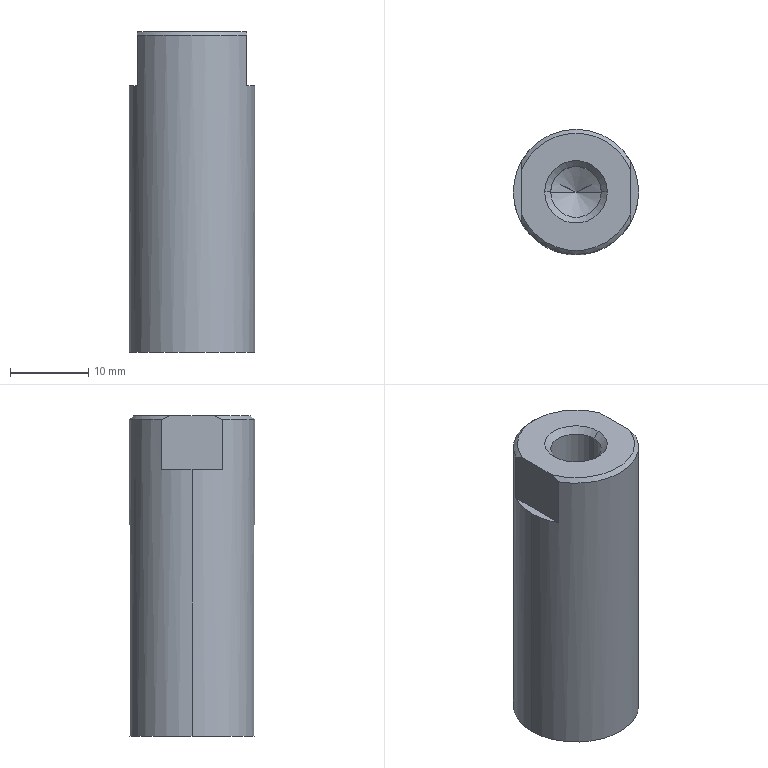Part | NX | features BREP 1 | 1 solid | 16 faces | box 16 x 16 x 41 mm | volume 7697 mm3 | cone 6 | plane 6 | cylinder 4 | commonest cylinder face diameters 6.47 x2 16 x2
STEP:
#1=CARTESIAN_POINT('',(7.,3.873,0.1));
#2=VERTEX_POINT('',#1);
#3=CARTESIAN_POINT('',(8.,0.,0.1));
#4=VERTEX_POINT('',#3);
#5=CARTESIAN_POINT('',(0.,0.,0.1));
#6=DIRECTION('',(0.,0.,-1.));
#7=DIRECTION('',(-1.,0.,0.));
#8=AXIS2_PLACEMENT_3D('',#5,#6,#7);
#9=CIRCLE('',#8,8.);
#10=EDGE_CURVE('',#2,#4,#9,.T.);
#11=ORIENTED_EDGE('',*,*,#10,.T.);
#12=CARTESIAN_POINT('',(8.,0.,-34.));
#13=VERTEX_POINT('',#12);
#14=CARTESIAN_POINT('',(8.,0.,-13.75));
#15=DIRECTION('',(0.,0.,-1.));
#16=VECTOR('',#15,1000.);
#17=LINE('',#14,#16);
#18=EDGE_CURVE('',#4,#13,#17,.T.);
#19=ORIENTED_EDGE('',*,*,#18,.T.);
#20=CARTESIAN_POINT('',(-8.,0.,-34.));
#21=VERTEX_POINT('',#20);
#22=CARTESIAN_POINT('',(0.,0.,-34.));
#23=DIRECTION('',(0.,0.,1.));
#24=DIRECTION('',(-1.,0.,0.));
#25=AXIS2_PLACEMENT_3D('',#22,#23,#24);
#26=CIRCLE('',#25,8.);
#27=EDGE_CURVE('',#13,#21,#26,.T.);
#28=ORIENTED_EDGE('',*,*,#27,.T.);
#29=CARTESIAN_POINT('',(-8.,0.,0.1));
#30=VERTEX_POINT('',#29);
#31=CARTESIAN_POINT('',(-8.,0.,-13.75));
#32=DIRECTION('',(0.,0.,-1.));
#33=VECTOR('',#32,1000.);
#34=LINE('',#31,#33);
#35=EDGE_CURVE('',#30,#21,#34,.T.);
#36=ORIENTED_EDGE('',*,*,#35,.F.);
#37=CARTESIAN_POINT('',(-7.,3.873,0.1));
#38=VERTEX_POINT('',#37);
#39=CARTESIAN_POINT('',(0.,0.,0.1));
#40=DIRECTION('',(0.,0.,-1.));
#41=DIRECTION('',(-1.,0.,0.));
#42=AXIS2_PLACEMENT_3D('',#39,#40,#41);
#43=CIRCLE('',#42,8.);
#44=EDGE_CURVE('',#30,#38,#43,.T.);
#45=ORIENTED_EDGE('',*,*,#44,.T.);
#46=CARTESIAN_POINT('',(-7.,3.873,6.5));
#47=VERTEX_POINT('',#46);
#48=CARTESIAN_POINT('',(-7.,3.873,-13.75));
#49=DIRECTION('',(0.,0.,1.));
#50=VECTOR('',#49,1000.);
#51=LINE('',#48,#50);
#52=EDGE_CURVE('',#38,#47,#51,.T.);
#53=ORIENTED_EDGE('',*,*,#52,.T.);
#54=CARTESIAN_POINT('',(7.,3.873,6.5));
#55=VERTEX_POINT('',#54);
#56=CARTESIAN_POINT('',(0.,0.,6.5));
#57=DIRECTION('',(0.,0.,-1.));
#58=DIRECTION('',(-1.,0.,0.));
#59=AXIS2_PLACEMENT_3D('',#56,#57,#58);
#60=CIRCLE('',#59,8.);
#61=EDGE_CURVE('',#47,#55,#60,.T.);
#62=ORIENTED_EDGE('',*,*,#61,.T.);
#63=CARTESIAN_POINT('',(7.,3.873,-13.75));
#64=DIRECTION('',(0.,0.,-1.));
#65=VECTOR('',#64,1000.);
#66=LINE('',#63,#65);
#67=EDGE_CURVE('',#55,#2,#66,.T.);
#68=ORIENTED_EDGE('',*,*,#67,.T.);
#69=EDGE_LOOP('',(#11,#19,#28,#36,#45,#53,#62,#68));
#70=FACE_BOUND('',#69,.T.);
#71=CARTESIAN_POINT('',(0.,0.,-13.75));
#72=DIRECTION('',(0.,0.,-1.));
#73=DIRECTION('',(-1.,0.,0.));
#74=AXIS2_PLACEMENT_3D('',#71,#72,#73);
#75=CYLINDRICAL_SURFACE('',#74,8.);
#76=ADVANCED_FACE('',(#70),#75,.T.);
#77=CARTESIAN_POINT('',(-3.235,0.,6.235));
#78=VERTEX_POINT('',#77);
#79=CARTESIAN_POINT('',(3.235,0.,6.235));
#80=VERTEX_POINT('',#79);
#81=CARTESIAN_POINT('',(0.,0.,6.235));
#82=DIRECTION('',(0.,0.,1.));
#83=DIRECTION('',(0.,1.,0.));
#84=AXIS2_PLACEMENT_3D('',#81,#82,#83);
#85=CIRCLE('',#84,3.235);
#86=EDGE_CURVE('',#78,#80,#85,.T.);
#87=ORIENTED_EDGE('',*,*,#86,.F.);
#88=CARTESIAN_POINT('',(-4.,0.,7.));
#89=VERTEX_POINT('',#88);
#90=CARTESIAN_POINT('',(-4.,0.,7.));
#91=DIRECTION('',(-0.7071,0.,0.7071));
#92=VECTOR('',#91,1000.);
#93=LINE('',#90,#92);
#94=EDGE_CURVE('',#89,#78,#93,.F.);
#95=ORIENTED_EDGE('',*,*,#94,.F.);
#96=CARTESIAN_POINT('',(4.,0.,7.));
#97=VERTEX_POINT('',#96);
#98=CARTESIAN_POINT('',(0.,0.,7.));
#99=DIRECTION('',(0.,0.,-1.));
#100=DIRECTION('',(1.,0.,0.));
#101=AXIS2_PLACEMENT_3D('',#98,#99,#100);
#102=CIRCLE('',#101,4.);
#103=EDGE_CURVE('',#97,#89,#102,.T.);
#104=ORIENTED_EDGE('',*,*,#103,.F.);
#105=CARTESIAN_POINT('',(4.,0.,7.));
#106=DIRECTION('',(0.7071,0.,0.7071));
#107=VECTOR('',#106,1000.);
#108=LINE('',#105,#107);
#109=EDGE_CURVE('',#97,#80,#108,.F.);
#110=ORIENTED_EDGE('',*,*,#109,.T.);
#111=EDGE_LOOP('',(#87,#95,#104,#110));
#112=FACE_BOUND('',#111,.T.);
#113=CARTESIAN_POINT('',(0.,0.,7.));
#114=DIRECTION('',(0.,0.,1.));
#115=DIRECTION('',(1.,0.,0.));
#116=AXIS2_PLACEMENT_3D('',#113,#114,#115);
#117=CONICAL_SURFACE('',#116,4.,0.7854);
#118=ADVANCED_FACE('',(#112),#117,.F.);
#119=ORIENTED_EDGE('',*,*,#86,.T.);
#120=CARTESIAN_POINT('',(3.235,0.,-6.5));
#121=VERTEX_POINT('',#120);
#122=CARTESIAN_POINT('',(3.235,0.,-0.1325));
#123=DIRECTION('',(0.,0.,-1.));
#124=VECTOR('',#123,1000.);
#125=LINE('',#122,#124);
#126=EDGE_CURVE('',#80,#121,#125,.T.);
#127=ORIENTED_EDGE('',*,*,#126,.T.);
#128=CARTESIAN_POINT('',(-3.235,0.,-6.5));
#129=VERTEX_POINT('',#128);
#130=CARTESIAN_POINT('',(0.,0.,-6.5));
#131=DIRECTION('',(0.,0.,1.));
#132=DIRECTION('',(-1.,0.,0.));
#133=AXIS2_PLACEMENT_3D('',#130,#131,#132);
#134=CIRCLE('',#133,3.235);
#135=EDGE_CURVE('',#129,#121,#134,.T.);
#136=ORIENTED_EDGE('',*,*,#135,.F.);
#137=CARTESIAN_POINT('',(-3.235,0.,-0.1325));
#138=DIRECTION('',(0.,0.,-1.));
#139=VECTOR('',#138,1000.);
#140=LINE('',#137,#139);
#141=EDGE_CURVE('',#78,#129,#140,.T.);
#142=ORIENTED_EDGE('',*,*,#141,.F.);
#143=EDGE_LOOP('',(#119,#127,#136,#142));
#144=FACE_BOUND('',#143,.T.);
#145=CARTESIAN_POINT('',(0.,0.,-0.1325));
#146=DIRECTION('',(0.,0.,-1.));
#147=DIRECTION('',(-1.,0.,0.));
#148=AXIS2_PLACEMENT_3D('',#145,#146,#147);
#149=CYLINDRICAL_SURFACE('',#148,3.235);
#150=ADVANCED_FACE('',(#144),#149,.F.);
#151=CARTESIAN_POINT('',(0.,0.,-8.368));
#152=VERTEX_POINT('',#151);
#153=CARTESIAN_POINT('',(3.235,0.,-6.5));
#154=DIRECTION('',(0.866,0.,0.5));
#155=VECTOR('',#154,1000.);
#156=LINE('',#153,#155);
#157=EDGE_CURVE('',#121,#152,#156,.F.);
#158=ORIENTED_EDGE('',*,*,#157,.T.);
#159=CARTESIAN_POINT('',(-3.235,0.,-6.5));
#160=DIRECTION('',(-0.866,0.,0.5));
#161=VECTOR('',#160,1000.);
#162=LINE('',#159,#161);
#163=EDGE_CURVE('',#129,#152,#162,.F.);
#164=ORIENTED_EDGE('',*,*,#163,.F.);
#165=ORIENTED_EDGE('',*,*,#135,.T.);
#166=EDGE_LOOP('',(#158,#164,#165));
#167=FACE_BOUND('',#166,.T.);
#168=CARTESIAN_POINT('',(0.,0.,-6.5));
#169=DIRECTION('',(0.,0.,1.));
#170=DIRECTION('',(1.,0.,0.));
#171=AXIS2_PLACEMENT_3D('',#168,#169,#170);
#172=CONICAL_SURFACE('',#171,3.235,1.047);
#173=ADVANCED_FACE('',(#167),#172,.F.);
#174=ORIENTED_EDGE('',*,*,#18,.F.);
#175=CARTESIAN_POINT('',(7.,-3.873,0.1));
#176=VERTEX_POINT('',#175);
#177=CARTESIAN_POINT('',(0.,0.,0.1));
#178=DIRECTION('',(0.,0.,-1.));
#179=DIRECTION('',(-1.,0.,0.));
#180=AXIS2_PLACEMENT_3D('',#177,#178,#179);
#181=CIRCLE('',#180,8.);
#182=EDGE_CURVE('',#4,#176,#181,.T.);
#183=ORIENTED_EDGE('',*,*,#182,.T.);
#184=CARTESIAN_POINT('',(7.,-3.873,6.5));
#185=VERTEX_POINT('',#184);
#186=CARTESIAN_POINT('',(7.,-3.873,-13.75));
#187=DIRECTION('',(0.,0.,1.));
#188=VECTOR('',#187,1000.);
#189=LINE('',#186,#188);
#190=EDGE_CURVE('',#176,#185,#189,.T.);
#191=ORIENTED_EDGE('',*,*,#190,.T.);
#192=CARTESIAN_POINT('',(-7.,-3.873,6.5));
#193=VERTEX_POINT('',#192);
#194=CARTESIAN_POINT('',(0.,0.,6.5));
#195=DIRECTION('',(0.,0.,-1.));
#196=DIRECTION('',(-1.,0.,0.));
#197=AXIS2_PLACEMENT_3D('',#194,#195,#196);
#198=CIRCLE('',#197,8.);
#199=EDGE_CURVE('',#185,#193,#198,.T.);
#200=ORIENTED_EDGE('',*,*,#199,.T.);
#201=CARTESIAN_POINT('',(-7.,-3.873,0.1));
#202=VERTEX_POINT('',#201);
#203=CARTESIAN_POINT('',(-7.,-3.873,-13.75));
#204=DIRECTION('',(0.,0.,-1.));
#205=VECTOR('',#204,1000.);
#206=LINE('',#203,#205);
#207=EDGE_CURVE('',#193,#202,#206,.T.);
#208=ORIENTED_EDGE('',*,*,#207,.T.);
#209=CARTESIAN_POINT('',(0.,0.,0.1));
#210=DIRECTION('',(0.,0.,-1.));
#211=DIRECTION('',(-1.,0.,0.));
#212=AXIS2_PLACEMENT_3D('',#209,#210,#211);
#213=CIRCLE('',#212,8.);
#214=EDGE_CURVE('',#202,#30,#213,.T.);
#215=ORIENTED_EDGE('',*,*,#214,.T.);
#216=ORIENTED_EDGE('',*,*,#35,.T.);
#217=CARTESIAN_POINT('',(0.,0.,-34.));
#218=DIRECTION('',(0.,0.,1.));
#219=DIRECTION('',(-1.,0.,0.));
#220=AXIS2_PLACEMENT_3D('',#217,#218,#219);
#221=CIRCLE('',#220,8.);
#222=EDGE_CURVE('',#21,#13,#221,.T.);
#223=ORIENTED_EDGE('',*,*,#222,.T.);
#224=EDGE_LOOP('',(#174,#183,#191,#200,#208,#215,#216,#223));
#225=FACE_BOUND('',#224,.T.);
#226=CARTESIAN_POINT('',(0.,0.,-13.75));
#227=DIRECTION('',(0.,0.,-1.));
#228=DIRECTION('',(-1.,0.,0.));
#229=AXIS2_PLACEMENT_3D('',#226,#227,#228);
#230=CYLINDRICAL_SURFACE('',#229,8.);
#231=ADVANCED_FACE('',(#225),#230,.T.);
#232=CARTESIAN_POINT('',(-7.,2.693,7.));
#233=VERTEX_POINT('',#232);
#234=CARTESIAN_POINT('',(-7.,2.693,7.));
#235=CARTESIAN_POINT('',(-7.,3.073,6.863));
#236=CARTESIAN_POINT('',(-7.,3.467,6.697));
#237=CARTESIAN_POINT('',(-7.,3.873,6.5));
#238=B_SPLINE_CURVE_WITH_KNOTS('',3,(#234,#235,#236,#237),.UNSPECIFIED.,.F.,.F.,(4,4),(0.,1.),.UNSPECIFIED.);
#239=EDGE_CURVE('',#47,#233,#238,.F.);
#240=ORIENTED_EDGE('',*,*,#239,.T.);
#241=CARTESIAN_POINT('',(7.,2.693,7.));
#242=VERTEX_POINT('',#241);
#243=CARTESIAN_POINT('',(0.,0.,7.));
#244=DIRECTION('',(0.,0.,-1.));
#245=DIRECTION('',(-1.,0.,0.));
#246=AXIS2_PLACEMENT_3D('',#243,#244,#245);
#247=CIRCLE('',#246,7.5);
#248=EDGE_CURVE('',#233,#242,#247,.T.);
#249=ORIENTED_EDGE('',*,*,#248,.T.);
#250=CARTESIAN_POINT('',(7.,3.873,6.5));
#251=CARTESIAN_POINT('',(7.,3.467,6.697));
#252=CARTESIAN_POINT('',(7.,3.073,6.863));
#253=CARTESIAN_POINT('',(7.,2.693,7.));
#254=B_SPLINE_CURVE_WITH_KNOTS('',3,(#250,#251,#252,#253),.UNSPECIFIED.,.F.,.F.,(4,4),(0.,1.),.UNSPECIFIED.);
#255=EDGE_CURVE('',#242,#55,#254,.F.);
#256=ORIENTED_EDGE('',*,*,#255,.T.);
#257=ORIENTED_EDGE('',*,*,#61,.F.);
#258=EDGE_LOOP('',(#240,#249,#256,#257));
#259=FACE_BOUND('',#258,.T.);
#260=CARTESIAN_POINT('',(0.,0.,6.5));
#261=DIRECTION('',(0.,0.,-1.));
#262=DIRECTION('',(-1.,0.,0.));
#263=AXIS2_PLACEMENT_3D('',#260,#261,#262);
#264=CONICAL_SURFACE('',#263,8.,0.7854);
#265=ADVANCED_FACE('',(#259),#264,.T.);
#266=CARTESIAN_POINT('',(-7.,-2.693,7.));
#267=VERTEX_POINT('',#266);
#268=CARTESIAN_POINT('',(-7.,-10.,7.));
#269=DIRECTION('',(0.,-1.,0.));
#270=VECTOR('',#269,1000.);
#271=LINE('',#268,#270);
#272=EDGE_CURVE('',#233,#267,#271,.T.);
#273=ORIENTED_EDGE('',*,*,#272,.F.);
#274=ORIENTED_EDGE('',*,*,#239,.F.);
#275=ORIENTED_EDGE('',*,*,#52,.F.);
#276=CARTESIAN_POINT('',(-7.,-10.,0.1));
#277=DIRECTION('',(0.,1.,0.));
#278=VECTOR('',#277,1000.);
#279=LINE('',#276,#278);
#280=EDGE_CURVE('',#202,#38,#279,.T.);
#281=ORIENTED_EDGE('',*,*,#280,.F.);
#282=ORIENTED_EDGE('',*,*,#207,.F.);
#283=CARTESIAN_POINT('',(-7.,-3.873,6.5));
#284=CARTESIAN_POINT('',(-7.,-3.467,6.697));
#285=CARTESIAN_POINT('',(-7.,-3.073,6.863));
#286=CARTESIAN_POINT('',(-7.,-2.693,7.));
#287=B_SPLINE_CURVE_WITH_KNOTS('',3,(#283,#284,#285,#286),.UNSPECIFIED.,.F.,.F.,(4,4),(0.,1.),.UNSPECIFIED.);
#288=EDGE_CURVE('',#267,#193,#287,.F.);
#289=ORIENTED_EDGE('',*,*,#288,.F.);
#290=EDGE_LOOP('',(#273,#274,#275,#281,#282,#289));
#291=FACE_BOUND('',#290,.T.);
#292=CARTESIAN_POINT('',(-7.,-10.,7.));
#293=DIRECTION('',(1.,0.,0.));
#294=DIRECTION('',(0.,1.,0.));
#295=AXIS2_PLACEMENT_3D('',#292,#293,#294);
#296=PLANE('',#295);
#297=ADVANCED_FACE('',(#291),#296,.F.);
#298=ORIENTED_EDGE('',*,*,#214,.F.);
#299=ORIENTED_EDGE('',*,*,#280,.T.);
#300=ORIENTED_EDGE('',*,*,#44,.F.);
#301=EDGE_LOOP('',(#298,#299,#300));
#302=FACE_BOUND('',#301,.T.);
#303=CARTESIAN_POINT('',(0.,0.,0.1));
#304=DIRECTION('',(0.,0.,1.));
#305=DIRECTION('',(1.,0.,0.));
#306=AXIS2_PLACEMENT_3D('',#303,#304,#305);
#307=PLANE('',#306);
#308=ADVANCED_FACE('',(#302),#307,.T.);
#309=ORIENTED_EDGE('',*,*,#288,.T.);
#310=ORIENTED_EDGE('',*,*,#199,.F.);
#311=CARTESIAN_POINT('',(7.,-2.693,7.));
#312=VERTEX_POINT('',#311);
#313=CARTESIAN_POINT('',(7.,-2.693,7.));
#314=CARTESIAN_POINT('',(7.,-3.073,6.863));
#315=CARTESIAN_POINT('',(7.,-3.467,6.697));
#316=CARTESIAN_POINT('',(7.,-3.873,6.5));
#317=B_SPLINE_CURVE_WITH_KNOTS('',3,(#313,#314,#315,#316),.UNSPECIFIED.,.F.,.F.,(4,4),(0.,1.),.UNSPECIFIED.);
#318=EDGE_CURVE('',#185,#312,#317,.F.);
#319=ORIENTED_EDGE('',*,*,#318,.T.);
#320=CARTESIAN_POINT('',(0.,0.,7.));
#321=DIRECTION('',(0.,0.,-1.));
#322=DIRECTION('',(-1.,0.,0.));
#323=AXIS2_PLACEMENT_3D('',#320,#321,#322);
#324=CIRCLE('',#323,7.5);
#325=EDGE_CURVE('',#312,#267,#324,.T.);
#326=ORIENTED_EDGE('',*,*,#325,.T.);
#327=EDGE_LOOP('',(#309,#310,#319,#326));
#328=FACE_BOUND('',#327,.T.);
#329=CARTESIAN_POINT('',(0.,0.,6.5));
#330=DIRECTION('',(0.,0.,-1.));
#331=DIRECTION('',(-1.,0.,0.));
#332=AXIS2_PLACEMENT_3D('',#329,#330,#331);
#333=CONICAL_SURFACE('',#332,8.,0.7854);
#334=ADVANCED_FACE('',(#328),#333,.T.);
#335=ORIENTED_EDGE('',*,*,#222,.F.);
#336=ORIENTED_EDGE('',*,*,#27,.F.);
#337=EDGE_LOOP('',(#335,#336));
#338=FACE_BOUND('',#337,.T.);
#339=CARTESIAN_POINT('',(0.,4.,-34.));
#340=DIRECTION('',(0.,0.,-1.));
#341=DIRECTION('',(0.,-1.,0.));
#342=AXIS2_PLACEMENT_3D('',#339,#340,#341);
#343=PLANE('',#342);
#344=ADVANCED_FACE('',(#338),#343,.T.);
#345=CARTESIAN_POINT('',(7.,3.75,7.));
#346=DIRECTION('',(0.,1.,0.));
#347=VECTOR('',#346,1000.);
#348=LINE('',#345,#347);
#349=EDGE_CURVE('',#312,#242,#348,.T.);
#350=ORIENTED_EDGE('',*,*,#349,.T.);
#351=ORIENTED_EDGE('',*,*,#248,.F.);
#352=ORIENTED_EDGE('',*,*,#272,.T.);
#353=ORIENTED_EDGE('',*,*,#325,.F.);
#354=EDGE_LOOP('',(#350,#351,#352,#353));
#355=FACE_BOUND('',#354,.T.);
#356=ORIENTED_EDGE('',*,*,#103,.T.);
#357=CARTESIAN_POINT('',(0.,0.,7.));
#358=DIRECTION('',(0.,0.,-1.));
#359=DIRECTION('',(1.,0.,0.));
#360=AXIS2_PLACEMENT_3D('',#357,#358,#359);
#361=CIRCLE('',#360,4.);
#362=EDGE_CURVE('',#89,#97,#361,.T.);
#363=ORIENTED_EDGE('',*,*,#362,.T.);
#364=EDGE_LOOP('',(#356,#363));
#365=FACE_BOUND('',#364,.T.);
#366=CARTESIAN_POINT('',(0.,3.75,7.));
#367=DIRECTION('',(0.,0.,1.));
#368=DIRECTION('',(1.,0.,0.));
#369=AXIS2_PLACEMENT_3D('',#366,#367,#368);
#370=PLANE('',#369);
#371=ADVANCED_FACE('',(#355,#365),#370,.T.);
#372=ORIENTED_EDGE('',*,*,#349,.F.);
#373=ORIENTED_EDGE('',*,*,#318,.F.);
#374=ORIENTED_EDGE('',*,*,#190,.F.);
#375=CARTESIAN_POINT('',(7.,10.,0.1));
#376=DIRECTION('',(0.,-1.,0.));
#377=VECTOR('',#376,1000.);
#378=LINE('',#375,#377);
#379=EDGE_CURVE('',#2,#176,#378,.T.);
#380=ORIENTED_EDGE('',*,*,#379,.F.);
#381=ORIENTED_EDGE('',*,*,#67,.F.);
#382=ORIENTED_EDGE('',*,*,#255,.F.);
#383=EDGE_LOOP('',(#372,#373,#374,#380,#381,#382));
#384=FACE_BOUND('',#383,.T.);
#385=CARTESIAN_POINT('',(7.,10.,7.));
#386=DIRECTION('',(-1.,0.,0.));
#387=DIRECTION('',(0.,0.,1.));
#388=AXIS2_PLACEMENT_3D('',#385,#386,#387);
#389=PLANE('',#388);
#390=ADVANCED_FACE('',(#384),#389,.F.);
#391=ORIENTED_EDGE('',*,*,#10,.F.);
#392=ORIENTED_EDGE('',*,*,#379,.T.);
#393=ORIENTED_EDGE('',*,*,#182,.F.);
#394=EDGE_LOOP('',(#391,#392,#393));
#395=FACE_BOUND('',#394,.T.);
#396=CARTESIAN_POINT('',(0.,0.,0.1));
#397=DIRECTION('',(0.,0.,1.));
#398=DIRECTION('',(1.,0.,0.));
#399=AXIS2_PLACEMENT_3D('',#396,#397,#398);
#400=PLANE('',#399);
#401=ADVANCED_FACE('',(#395),#400,.T.);
#402=ORIENTED_EDGE('',*,*,#94,.T.);
#403=CARTESIAN_POINT('',(0.,0.,6.235));
#404=DIRECTION('',(0.,0.,1.));
#405=DIRECTION('',(0.,1.,0.));
#406=AXIS2_PLACEMENT_3D('',#403,#404,#405);
#407=CIRCLE('',#406,3.235);
#408=EDGE_CURVE('',#80,#78,#407,.T.);
#409=ORIENTED_EDGE('',*,*,#408,.F.);
#410=ORIENTED_EDGE('',*,*,#109,.F.);
#411=ORIENTED_EDGE('',*,*,#362,.F.);
#412=EDGE_LOOP('',(#402,#409,#410,#411));
#413=FACE_BOUND('',#412,.T.);
#414=CARTESIAN_POINT('',(0.,0.,7.));
#415=DIRECTION('',(0.,0.,1.));
#416=DIRECTION('',(1.,0.,0.));
#417=AXIS2_PLACEMENT_3D('',#414,#415,#416);
#418=CONICAL_SURFACE('',#417,4.,0.7854);
#419=ADVANCED_FACE('',(#413),#418,.F.);
#420=ORIENTED_EDGE('',*,*,#126,.F.);
#421=ORIENTED_EDGE('',*,*,#408,.T.);
#422=ORIENTED_EDGE('',*,*,#141,.T.);
#423=CARTESIAN_POINT('',(0.,0.,-6.5));
#424=DIRECTION('',(0.,0.,1.));
#425=DIRECTION('',(-1.,0.,0.));
#426=AXIS2_PLACEMENT_3D('',#423,#424,#425);
#427=CIRCLE('',#426,3.235);
#428=EDGE_CURVE('',#121,#129,#427,.T.);
#429=ORIENTED_EDGE('',*,*,#428,.F.);
#430=EDGE_LOOP('',(#420,#421,#422,#429));
#431=FACE_BOUND('',#430,.T.);
#432=CARTESIAN_POINT('',(0.,0.,-0.1325));
#433=DIRECTION('',(0.,0.,-1.));
#434=DIRECTION('',(-1.,0.,0.));
#435=AXIS2_PLACEMENT_3D('',#432,#433,#434);
#436=CYLINDRICAL_SURFACE('',#435,3.235);
#437=ADVANCED_FACE('',(#431),#436,.F.);
#438=ORIENTED_EDGE('',*,*,#163,.T.);
#439=ORIENTED_EDGE('',*,*,#157,.F.);
#440=ORIENTED_EDGE('',*,*,#428,.T.);
#441=EDGE_LOOP('',(#438,#439,#440));
#442=FACE_BOUND('',#441,.T.);
#443=CARTESIAN_POINT('',(0.,0.,-6.5));
#444=DIRECTION('',(0.,0.,1.));
#445=DIRECTION('',(1.,0.,0.));
#446=AXIS2_PLACEMENT_3D('',#443,#444,#445);
#447=CONICAL_SURFACE('',#446,3.235,1.047);
#448=ADVANCED_FACE('',(#442),#447,.F.);
#449=CLOSED_SHELL('',(#76,#118,#150,#173,#231,#265,#297,#308,#334,#344,#371,#390,#401,#419,#437,#448));
#450=MANIFOLD_SOLID_BREP('',#449);
#451=(LENGTH_UNIT()NAMED_UNIT(*)SI_UNIT(.MILLI.,.METRE.));
#452=UNCERTAINTY_MEASURE_WITH_UNIT(LENGTH_MEASURE(0.0508),#451,'','');
#453=(NAMED_UNIT(*)PLANE_ANGLE_UNIT()SI_UNIT($,.RADIAN.));
#454=(NAMED_UNIT(*)SI_UNIT($,.STERADIAN.)SOLID_ANGLE_UNIT());
#455=(GEOMETRIC_REPRESENTATION_CONTEXT(3)GLOBAL_UNCERTAINTY_ASSIGNED_CONTEXT((#452))GLOBAL_UNIT_ASSIGNED_CONTEXT((#451,#453,#454))REPRESENTATION_CONTEXT('',''));
#456=ADVANCED_BREP_SHAPE_REPRESENTATION('',(#450),#455);